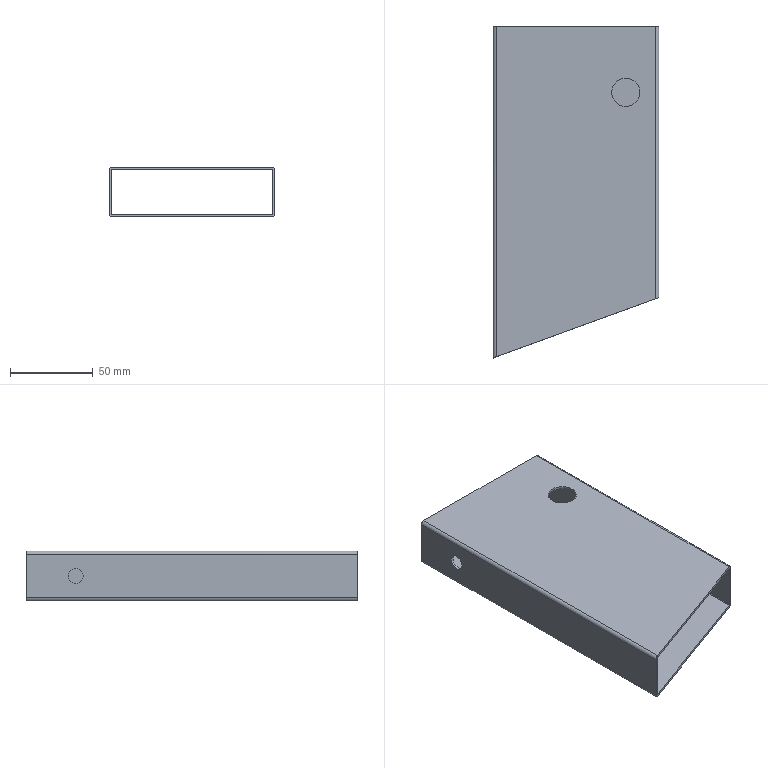Part | STEP file | PN_0060 | 1 solid | 23 faces | box 100 x 200 x 30 mm | volume 68036 mm3 | cylinder 13 | plane 10 | commonest cylinder face diameters 4 x5 1 x4 9 x3 17 x1